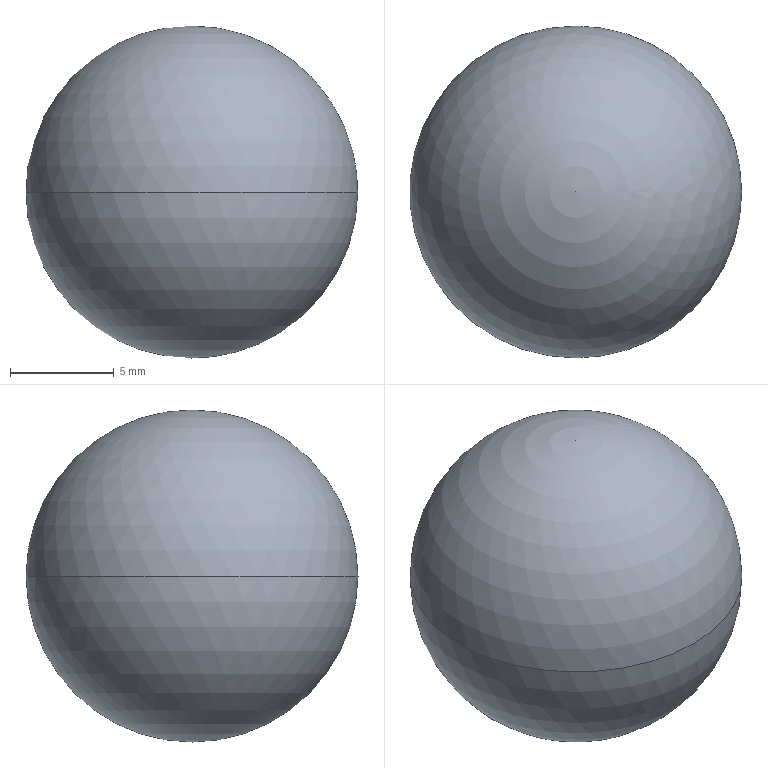Part | SolidWorks | features Revolution 1 | 1 solid | 2 faces | box 16 x 16 x 16 mm | volume 2145 mm3 | sphere 2
STEP:
#1=CARTESIAN_POINT('',(0.,-8.,0.));
#2=VERTEX_POINT('',#1);
#3=CARTESIAN_POINT('',(0.,8.,0.));
#4=VERTEX_POINT('',#3);
#5=CARTESIAN_POINT('',(0.,0.,0.));
#6=DIRECTION('',(0.,0.,1.));
#7=DIRECTION('',(1.,0.,0.));
#8=AXIS2_PLACEMENT_3D('',#5,#6,#7);
#9=CIRCLE('',#8,8.);
#10=EDGE_CURVE('',#2,#4,#9,.T.);
#11=ORIENTED_EDGE('',*,*,#10,.F.);
#12=CARTESIAN_POINT('',(0.,0.,0.));
#13=DIRECTION('',(0.,0.,-1.));
#14=DIRECTION('',(-1.,0.,0.));
#15=AXIS2_PLACEMENT_3D('',#12,#13,#14);
#16=CIRCLE('',#15,8.);
#17=EDGE_CURVE('',#2,#4,#16,.T.);
#18=ORIENTED_EDGE('',*,*,#17,.T.);
#19=EDGE_LOOP('',(#11,#18));
#20=FACE_OUTER_BOUND('',#19,.T.);
#21=CARTESIAN_POINT('',(0.,0.,0.));
#22=DIRECTION('',(0.,0.,-1.));
#23=DIRECTION('',(1.,0.,0.));
#24=AXIS2_PLACEMENT_3D('',#21,#22,#23);
#25=SPHERICAL_SURFACE('',#24,8.);
#26=ADVANCED_FACE('',(#20),#25,.T.);
#27=ORIENTED_EDGE('',*,*,#17,.F.);
#28=ORIENTED_EDGE('',*,*,#10,.T.);
#29=EDGE_LOOP('',(#27,#28));
#30=FACE_OUTER_BOUND('',#29,.T.);
#31=CARTESIAN_POINT('',(0.,0.,0.));
#32=DIRECTION('',(0.,0.,-1.));
#33=DIRECTION('',(1.,0.,0.));
#34=AXIS2_PLACEMENT_3D('',#31,#32,#33);
#35=SPHERICAL_SURFACE('',#34,8.);
#36=ADVANCED_FACE('',(#30),#35,.T.);
#37=CLOSED_SHELL('',(#26,#36));
#38=MANIFOLD_SOLID_BREP('',#37);
#39=CARTESIAN_POINT('',(0.,0.,0.));
#40=DIRECTION('',(0.,0.,1.));
#41=DIRECTION('',(1.,0.,0.));
#42=AXIS2_PLACEMENT_3D('',#39,#40,#41);
#43=(LENGTH_UNIT()NAMED_UNIT(*)SI_UNIT(.MILLI.,.METRE.));
#44=UNCERTAINTY_MEASURE_WITH_UNIT(LENGTH_MEASURE(0.00001),#43,'','');
#45=(NAMED_UNIT(*)PLANE_ANGLE_UNIT()SI_UNIT($,.RADIAN.));
#46=(NAMED_UNIT(*)SI_UNIT($,.STERADIAN.)SOLID_ANGLE_UNIT());
#47=(GEOMETRIC_REPRESENTATION_CONTEXT(3)GLOBAL_UNCERTAINTY_ASSIGNED_CONTEXT((#44))GLOBAL_UNIT_ASSIGNED_CONTEXT((#43,#45,#46))REPRESENTATION_CONTEXT('',''));
#48=ADVANCED_BREP_SHAPE_REPRESENTATION('',(#38,#42),#47);